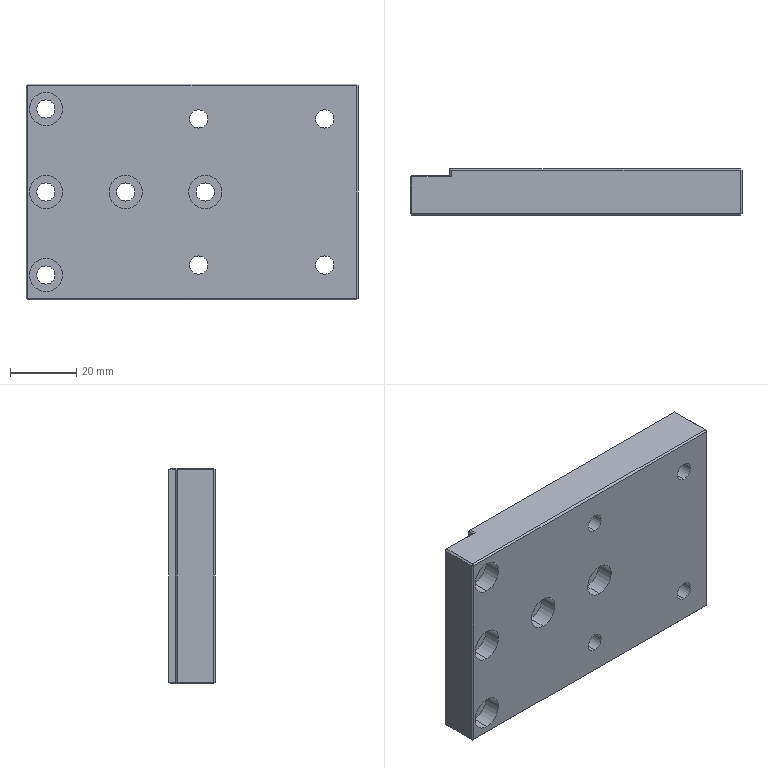Part | STEP file | ND25021-01-JDKM-63-TL | 1 solid | 77 faces | box 100 x 14 x 65 mm | volume 83838 mm3 | plane 41 | cylinder 36 | commonest cylinder face diameters 5.5 x18 10 x18